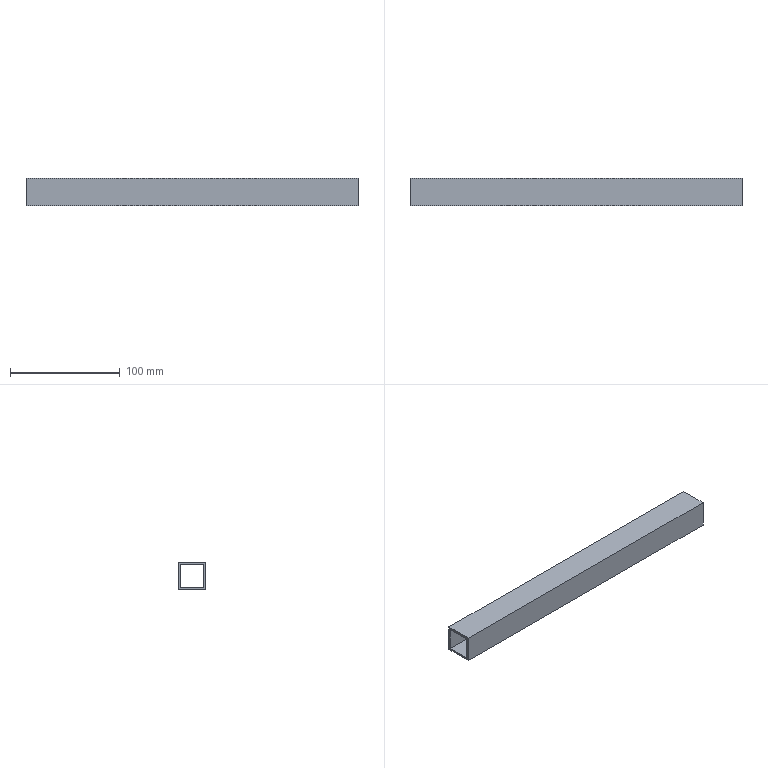Part | NX | features solid 2 | 1 solid | 10 faces | box 302.5 x 25 x 25 mm | volume 55660 mm3 | plane 10
STEP:
#1=CARTESIAN_POINT('',(487.5,292.5,-15.));
#2=VERTEX_POINT('',#1);
#3=CARTESIAN_POINT('',(487.5,267.5,-15.));
#4=VERTEX_POINT('',#3);
#5=CARTESIAN_POINT('',(487.5,145.,-15.));
#6=DIRECTION('',(0.,1.,0.));
#7=VECTOR('',#6,1000.);
#8=LINE('',#5,#7);
#9=EDGE_CURVE('',#2,#4,#8,.F.);
#10=ORIENTED_EDGE('',*,*,#9,.F.);
#11=CARTESIAN_POINT('',(487.5,292.5,10.));
#12=VERTEX_POINT('',#11);
#13=CARTESIAN_POINT('',(487.5,292.5,-10.));
#14=DIRECTION('',(0.,0.,1.));
#15=VECTOR('',#14,1000.);
#16=LINE('',#13,#15);
#17=EDGE_CURVE('',#2,#12,#16,.T.);
#18=ORIENTED_EDGE('',*,*,#17,.T.);
#19=CARTESIAN_POINT('',(487.5,267.5,10.));
#20=VERTEX_POINT('',#19);
#21=CARTESIAN_POINT('',(487.5,515.,10.));
#22=DIRECTION('',(0.,1.,0.));
#23=VECTOR('',#22,1000.);
#24=LINE('',#21,#23);
#25=EDGE_CURVE('',#12,#20,#24,.F.);
#26=ORIENTED_EDGE('',*,*,#25,.T.);
#27=CARTESIAN_POINT('',(487.5,267.5,-10.));
#28=DIRECTION('',(0.,0.,1.));
#29=VECTOR('',#28,1000.);
#30=LINE('',#27,#29);
#31=EDGE_CURVE('',#4,#20,#30,.T.);
#32=ORIENTED_EDGE('',*,*,#31,.F.);
#33=EDGE_LOOP('',(#10,#18,#26,#32));
#34=FACE_BOUND('',#33,.T.);
#35=CARTESIAN_POINT('',(487.5,290.5,-13.));
#36=VERTEX_POINT('',#35);
#37=CARTESIAN_POINT('',(487.5,269.5,-13.));
#38=VERTEX_POINT('',#37);
#39=CARTESIAN_POINT('',(487.5,145.,-13.));
#40=DIRECTION('',(0.,1.,0.));
#41=VECTOR('',#40,1000.);
#42=LINE('',#39,#41);
#43=EDGE_CURVE('',#36,#38,#42,.F.);
#44=ORIENTED_EDGE('',*,*,#43,.T.);
#45=CARTESIAN_POINT('',(487.5,269.5,8.));
#46=VERTEX_POINT('',#45);
#47=CARTESIAN_POINT('',(487.5,269.5,-10.));
#48=DIRECTION('',(0.,0.,1.));
#49=VECTOR('',#48,1000.);
#50=LINE('',#47,#49);
#51=EDGE_CURVE('',#38,#46,#50,.T.);
#52=ORIENTED_EDGE('',*,*,#51,.T.);
#53=CARTESIAN_POINT('',(487.5,290.5,8.));
#54=VERTEX_POINT('',#53);
#55=CARTESIAN_POINT('',(487.5,515.,8.));
#56=DIRECTION('',(0.,1.,0.));
#57=VECTOR('',#56,1000.);
#58=LINE('',#55,#57);
#59=EDGE_CURVE('',#54,#46,#58,.F.);
#60=ORIENTED_EDGE('',*,*,#59,.F.);
#61=CARTESIAN_POINT('',(487.5,290.5,-10.));
#62=DIRECTION('',(0.,0.,1.));
#63=VECTOR('',#62,1000.);
#64=LINE('',#61,#63);
#65=EDGE_CURVE('',#36,#54,#64,.T.);
#66=ORIENTED_EDGE('',*,*,#65,.F.);
#67=EDGE_LOOP('',(#44,#52,#60,#66));
#68=FACE_BOUND('',#67,.T.);
#69=CARTESIAN_POINT('',(487.5,145.,5.));
#70=DIRECTION('',(-1.,0.,0.));
#71=DIRECTION('',(0.,0.,1.));
#72=AXIS2_PLACEMENT_3D('',#69,#70,#71);
#73=PLANE('',#72);
#74=ADVANCED_FACE('',(#34,#68),#73,.F.);
#75=CARTESIAN_POINT('',(185.,292.5,-15.));
#76=VERTEX_POINT('',#75);
#77=CARTESIAN_POINT('',(-22.5,292.5,-15.));
#78=DIRECTION('',(-1.,0.,0.));
#79=VECTOR('',#78,1000.);
#80=LINE('',#77,#79);
#81=EDGE_CURVE('',#76,#2,#80,.F.);
#82=ORIENTED_EDGE('',*,*,#81,.T.);
#83=ORIENTED_EDGE('',*,*,#9,.T.);
#84=CARTESIAN_POINT('',(185.,267.5,-15.));
#85=VERTEX_POINT('',#84);
#86=CARTESIAN_POINT('',(-22.5,267.5,-15.));
#87=DIRECTION('',(-1.,0.,0.));
#88=VECTOR('',#87,1000.);
#89=LINE('',#86,#88);
#90=EDGE_CURVE('',#85,#4,#89,.F.);
#91=ORIENTED_EDGE('',*,*,#90,.F.);
#92=CARTESIAN_POINT('',(185.,-125.,-15.));
#93=DIRECTION('',(0.,1.,0.));
#94=VECTOR('',#93,1000.);
#95=LINE('',#92,#94);
#96=EDGE_CURVE('',#76,#85,#95,.F.);
#97=ORIENTED_EDGE('',*,*,#96,.F.);
#98=EDGE_LOOP('',(#82,#83,#91,#97));
#99=FACE_BOUND('',#98,.T.);
#100=CARTESIAN_POINT('',(212.5,-125.,-15.));
#101=DIRECTION('',(0.,0.,-1.));
#102=DIRECTION('',(-1.,0.,0.));
#103=AXIS2_PLACEMENT_3D('',#100,#101,#102);
#104=PLANE('',#103);
#105=ADVANCED_FACE('',(#99),#104,.T.);
#106=CARTESIAN_POINT('',(185.,267.5,10.));
#107=VERTEX_POINT('',#106);
#108=CARTESIAN_POINT('',(255.,267.5,10.));
#109=DIRECTION('',(-1.,0.,0.));
#110=VECTOR('',#109,1000.);
#111=LINE('',#108,#110);
#112=EDGE_CURVE('',#107,#20,#111,.F.);
#113=ORIENTED_EDGE('',*,*,#112,.T.);
#114=ORIENTED_EDGE('',*,*,#25,.F.);
#115=CARTESIAN_POINT('',(185.,292.5,10.));
#116=VERTEX_POINT('',#115);
#117=CARTESIAN_POINT('',(255.,292.5,10.));
#118=DIRECTION('',(-1.,0.,0.));
#119=VECTOR('',#118,1000.);
#120=LINE('',#117,#119);
#121=EDGE_CURVE('',#116,#12,#120,.F.);
#122=ORIENTED_EDGE('',*,*,#121,.F.);
#123=CARTESIAN_POINT('',(185.,515.,10.));
#124=DIRECTION('',(0.,-1.,0.));
#125=VECTOR('',#124,1000.);
#126=LINE('',#123,#125);
#127=EDGE_CURVE('',#107,#116,#126,.F.);
#128=ORIENTED_EDGE('',*,*,#127,.F.);
#129=EDGE_LOOP('',(#113,#114,#122,#128));
#130=FACE_BOUND('',#129,.T.);
#131=CARTESIAN_POINT('',(255.,515.,10.));
#132=DIRECTION('',(0.,0.,1.));
#133=DIRECTION('',(0.,-1.,0.));
#134=AXIS2_PLACEMENT_3D('',#131,#132,#133);
#135=PLANE('',#134);
#136=ADVANCED_FACE('',(#130),#135,.T.);
#137=CARTESIAN_POINT('',(185.,267.5,-10.));
#138=DIRECTION('',(0.,0.,-1.));
#139=VECTOR('',#138,1000.);
#140=LINE('',#137,#139);
#141=EDGE_CURVE('',#107,#85,#140,.T.);
#142=ORIENTED_EDGE('',*,*,#141,.T.);
#143=ORIENTED_EDGE('',*,*,#90,.T.);
#144=ORIENTED_EDGE('',*,*,#31,.T.);
#145=ORIENTED_EDGE('',*,*,#112,.F.);
#146=EDGE_LOOP('',(#142,#143,#144,#145));
#147=FACE_BOUND('',#146,.T.);
#148=CARTESIAN_POINT('',(-22.5,267.5,-10.));
#149=DIRECTION('',(0.,-1.,0.));
#150=DIRECTION('',(0.,0.,-1.));
#151=AXIS2_PLACEMENT_3D('',#148,#149,#150);
#152=PLANE('',#151);
#153=ADVANCED_FACE('',(#147),#152,.T.);
#154=ORIENTED_EDGE('',*,*,#121,.T.);
#155=ORIENTED_EDGE('',*,*,#17,.F.);
#156=ORIENTED_EDGE('',*,*,#81,.F.);
#157=CARTESIAN_POINT('',(185.,292.5,-10.));
#158=DIRECTION('',(0.,0.,-1.));
#159=VECTOR('',#158,1000.);
#160=LINE('',#157,#159);
#161=EDGE_CURVE('',#116,#76,#160,.T.);
#162=ORIENTED_EDGE('',*,*,#161,.F.);
#163=EDGE_LOOP('',(#154,#155,#156,#162));
#164=FACE_BOUND('',#163,.T.);
#165=CARTESIAN_POINT('',(-22.5,292.5,-10.));
#166=DIRECTION('',(0.,-1.,0.));
#167=DIRECTION('',(0.,0.,-1.));
#168=AXIS2_PLACEMENT_3D('',#165,#166,#167);
#169=PLANE('',#168);
#170=ADVANCED_FACE('',(#164),#169,.F.);
#171=CARTESIAN_POINT('',(185.,290.5,-13.));
#172=VERTEX_POINT('',#171);
#173=CARTESIAN_POINT('',(185.,269.5,-13.));
#174=VERTEX_POINT('',#173);
#175=CARTESIAN_POINT('',(185.,-125.,-13.));
#176=DIRECTION('',(0.,1.,0.));
#177=VECTOR('',#176,1000.);
#178=LINE('',#175,#177);
#179=EDGE_CURVE('',#172,#174,#178,.F.);
#180=ORIENTED_EDGE('',*,*,#179,.T.);
#181=CARTESIAN_POINT('',(-22.5,269.5,-13.));
#182=DIRECTION('',(-1.,0.,0.));
#183=VECTOR('',#182,1000.);
#184=LINE('',#181,#183);
#185=EDGE_CURVE('',#174,#38,#184,.F.);
#186=ORIENTED_EDGE('',*,*,#185,.T.);
#187=ORIENTED_EDGE('',*,*,#43,.F.);
#188=CARTESIAN_POINT('',(-22.5,290.5,-13.));
#189=DIRECTION('',(-1.,0.,0.));
#190=VECTOR('',#189,1000.);
#191=LINE('',#188,#190);
#192=EDGE_CURVE('',#172,#36,#191,.F.);
#193=ORIENTED_EDGE('',*,*,#192,.F.);
#194=EDGE_LOOP('',(#180,#186,#187,#193));
#195=FACE_BOUND('',#194,.T.);
#196=CARTESIAN_POINT('',(212.5,-125.,-13.));
#197=DIRECTION('',(0.,0.,-1.));
#198=DIRECTION('',(-1.,0.,0.));
#199=AXIS2_PLACEMENT_3D('',#196,#197,#198);
#200=PLANE('',#199);
#201=ADVANCED_FACE('',(#195),#200,.F.);
#202=CARTESIAN_POINT('',(185.,269.5,8.));
#203=VERTEX_POINT('',#202);
#204=CARTESIAN_POINT('',(185.,290.5,8.));
#205=VERTEX_POINT('',#204);
#206=CARTESIAN_POINT('',(185.,515.,8.));
#207=DIRECTION('',(0.,-1.,0.));
#208=VECTOR('',#207,1000.);
#209=LINE('',#206,#208);
#210=EDGE_CURVE('',#203,#205,#209,.F.);
#211=ORIENTED_EDGE('',*,*,#210,.T.);
#212=CARTESIAN_POINT('',(255.,290.5,8.));
#213=DIRECTION('',(-1.,0.,0.));
#214=VECTOR('',#213,1000.);
#215=LINE('',#212,#214);
#216=EDGE_CURVE('',#205,#54,#215,.F.);
#217=ORIENTED_EDGE('',*,*,#216,.T.);
#218=ORIENTED_EDGE('',*,*,#59,.T.);
#219=CARTESIAN_POINT('',(255.,269.5,8.));
#220=DIRECTION('',(-1.,0.,0.));
#221=VECTOR('',#220,1000.);
#222=LINE('',#219,#221);
#223=EDGE_CURVE('',#203,#46,#222,.F.);
#224=ORIENTED_EDGE('',*,*,#223,.F.);
#225=EDGE_LOOP('',(#211,#217,#218,#224));
#226=FACE_BOUND('',#225,.T.);
#227=CARTESIAN_POINT('',(255.,515.,8.));
#228=DIRECTION('',(0.,0.,1.));
#229=DIRECTION('',(0.,-1.,0.));
#230=AXIS2_PLACEMENT_3D('',#227,#228,#229);
#231=PLANE('',#230);
#232=ADVANCED_FACE('',(#226),#231,.F.);
#233=ORIENTED_EDGE('',*,*,#223,.T.);
#234=ORIENTED_EDGE('',*,*,#51,.F.);
#235=ORIENTED_EDGE('',*,*,#185,.F.);
#236=CARTESIAN_POINT('',(185.,269.5,-10.));
#237=DIRECTION('',(0.,0.,-1.));
#238=VECTOR('',#237,1000.);
#239=LINE('',#236,#238);
#240=EDGE_CURVE('',#203,#174,#239,.T.);
#241=ORIENTED_EDGE('',*,*,#240,.F.);
#242=EDGE_LOOP('',(#233,#234,#235,#241));
#243=FACE_BOUND('',#242,.T.);
#244=CARTESIAN_POINT('',(-22.5,269.5,-10.));
#245=DIRECTION('',(0.,-1.,0.));
#246=DIRECTION('',(0.,0.,-1.));
#247=AXIS2_PLACEMENT_3D('',#244,#245,#246);
#248=PLANE('',#247);
#249=ADVANCED_FACE('',(#243),#248,.F.);
#250=CARTESIAN_POINT('',(185.,290.5,-10.));
#251=DIRECTION('',(0.,0.,-1.));
#252=VECTOR('',#251,1000.);
#253=LINE('',#250,#252);
#254=EDGE_CURVE('',#205,#172,#253,.T.);
#255=ORIENTED_EDGE('',*,*,#254,.T.);
#256=ORIENTED_EDGE('',*,*,#192,.T.);
#257=ORIENTED_EDGE('',*,*,#65,.T.);
#258=ORIENTED_EDGE('',*,*,#216,.F.);
#259=EDGE_LOOP('',(#255,#256,#257,#258));
#260=FACE_BOUND('',#259,.T.);
#261=CARTESIAN_POINT('',(-22.5,290.5,-10.));
#262=DIRECTION('',(0.,-1.,0.));
#263=DIRECTION('',(0.,0.,-1.));
#264=AXIS2_PLACEMENT_3D('',#261,#262,#263);
#265=PLANE('',#264);
#266=ADVANCED_FACE('',(#260),#265,.T.);
#267=ORIENTED_EDGE('',*,*,#141,.F.);
#268=ORIENTED_EDGE('',*,*,#127,.T.);
#269=ORIENTED_EDGE('',*,*,#161,.T.);
#270=ORIENTED_EDGE('',*,*,#96,.T.);
#271=EDGE_LOOP('',(#267,#268,#269,#270));
#272=FACE_BOUND('',#271,.T.);
#273=ORIENTED_EDGE('',*,*,#210,.F.);
#274=ORIENTED_EDGE('',*,*,#240,.T.);
#275=ORIENTED_EDGE('',*,*,#179,.F.);
#276=ORIENTED_EDGE('',*,*,#254,.F.);
#277=EDGE_LOOP('',(#273,#274,#275,#276));
#278=FACE_BOUND('',#277,.T.);
#279=CARTESIAN_POINT('',(185.,-537.5,20.));
#280=DIRECTION('',(1.,0.,0.));
#281=DIRECTION('',(0.,0.,-1.));
#282=AXIS2_PLACEMENT_3D('',#279,#280,#281);
#283=PLANE('',#282);
#284=ADVANCED_FACE('',(#272,#278),#283,.F.);
#285=CLOSED_SHELL('',(#74,#105,#136,#153,#170,#201,#232,#249,#266,#284));
#286=MANIFOLD_SOLID_BREP('',#285);
#287=(LENGTH_UNIT()NAMED_UNIT(*)SI_UNIT(.MILLI.,.METRE.));
#288=UNCERTAINTY_MEASURE_WITH_UNIT(LENGTH_MEASURE(0.00001),#287,'','');
#289=(NAMED_UNIT(*)PLANE_ANGLE_UNIT()SI_UNIT($,.RADIAN.));
#290=(NAMED_UNIT(*)SI_UNIT($,.STERADIAN.)SOLID_ANGLE_UNIT());
#291=(GEOMETRIC_REPRESENTATION_CONTEXT(3)GLOBAL_UNCERTAINTY_ASSIGNED_CONTEXT((#288))GLOBAL_UNIT_ASSIGNED_CONTEXT((#287,#289,#290))REPRESENTATION_CONTEXT('',''));
#292=ADVANCED_BREP_SHAPE_REPRESENTATION('',(#286),#291);